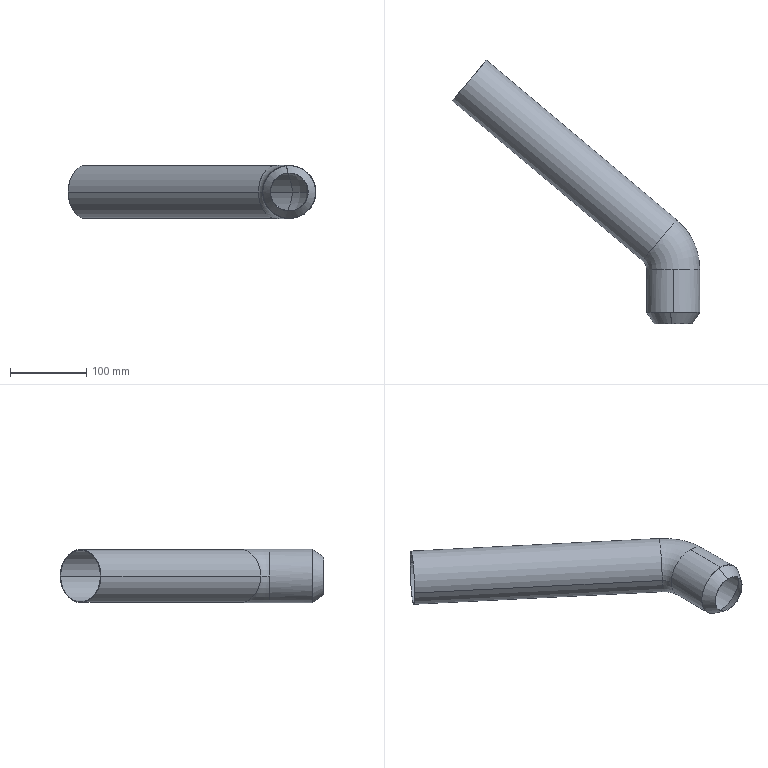Part | SolidWorks | features ICE 1, LoftedBend 1, Sweep 1, SweepCut 1 | 2 solids | 20 faces | box 325.613 x 346.787 x 70 mm | volume 94246 mm3 | cylinder 8 | spline 6 | torus 4 | plane 2 | commonest cylinder face diameters 68 x4 70 x4